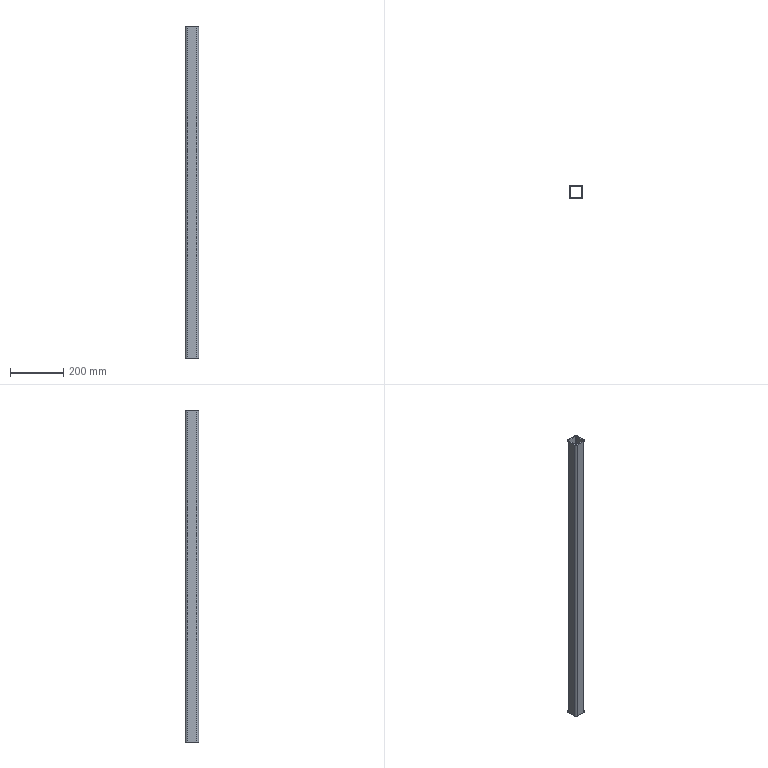Part | SolidWorks | features Extrusion 1 | 1 solid | 18 faces | box 50 x 50 x 1250 mm | volume 868496 mm3 | plane 10 | cylinder 8 | commonest cylinder face diameters 8 x4 16 x4
STEP:
#1=CARTESIAN_POINT('',(17.,-25.,625.));
#2=VERTEX_POINT('',#1);
#3=CARTESIAN_POINT('',(25.,-17.,625.));
#4=VERTEX_POINT('',#3);
#5=CARTESIAN_POINT('',(17.,-17.,625.));
#6=DIRECTION('',(0.,0.,1.));
#7=DIRECTION('',(1.,0.,0.));
#8=AXIS2_PLACEMENT_3D('',#5,#6,#7);
#9=CIRCLE('',#8,8.);
#10=EDGE_CURVE('',#2,#4,#9,.T.);
#11=ORIENTED_EDGE('',*,*,#10,.T.);
#12=CARTESIAN_POINT('',(25.,17.,625.));
#13=VERTEX_POINT('',#12);
#14=CARTESIAN_POINT('',(25.,-17.,625.));
#15=DIRECTION('',(0.,1.,0.));
#16=VECTOR('',#15,1000.);
#17=LINE('',#14,#16);
#18=EDGE_CURVE('',#4,#13,#17,.T.);
#19=ORIENTED_EDGE('',*,*,#18,.T.);
#20=CARTESIAN_POINT('',(17.,25.,625.));
#21=VERTEX_POINT('',#20);
#22=CARTESIAN_POINT('',(17.,17.,625.));
#23=DIRECTION('',(0.,0.,1.));
#24=DIRECTION('',(-1.,0.,0.));
#25=AXIS2_PLACEMENT_3D('',#22,#23,#24);
#26=CIRCLE('',#25,8.);
#27=EDGE_CURVE('',#13,#21,#26,.T.);
#28=ORIENTED_EDGE('',*,*,#27,.T.);
#29=CARTESIAN_POINT('',(-17.,25.,625.));
#30=VERTEX_POINT('',#29);
#31=CARTESIAN_POINT('',(-17.,25.,625.));
#32=DIRECTION('',(-1.,0.,0.));
#33=VECTOR('',#32,1000.);
#34=LINE('',#31,#33);
#35=EDGE_CURVE('',#21,#30,#34,.T.);
#36=ORIENTED_EDGE('',*,*,#35,.T.);
#37=CARTESIAN_POINT('',(-25.,17.,625.));
#38=VERTEX_POINT('',#37);
#39=CARTESIAN_POINT('',(-17.,17.,625.));
#40=DIRECTION('',(0.,0.,1.));
#41=DIRECTION('',(-1.,0.,0.));
#42=AXIS2_PLACEMENT_3D('',#39,#40,#41);
#43=CIRCLE('',#42,8.);
#44=EDGE_CURVE('',#30,#38,#43,.T.);
#45=ORIENTED_EDGE('',*,*,#44,.T.);
#46=CARTESIAN_POINT('',(-25.,-17.,625.));
#47=VERTEX_POINT('',#46);
#48=CARTESIAN_POINT('',(-25.,-17.,625.));
#49=DIRECTION('',(0.,-1.,0.));
#50=VECTOR('',#49,1000.);
#51=LINE('',#48,#50);
#52=EDGE_CURVE('',#38,#47,#51,.T.);
#53=ORIENTED_EDGE('',*,*,#52,.T.);
#54=CARTESIAN_POINT('',(-17.,-25.,625.));
#55=VERTEX_POINT('',#54);
#56=CARTESIAN_POINT('',(-17.,-17.,625.));
#57=DIRECTION('',(0.,0.,1.));
#58=DIRECTION('',(-1.,0.,0.));
#59=AXIS2_PLACEMENT_3D('',#56,#57,#58);
#60=CIRCLE('',#59,8.);
#61=EDGE_CURVE('',#47,#55,#60,.T.);
#62=ORIENTED_EDGE('',*,*,#61,.T.);
#63=CARTESIAN_POINT('',(-17.,-25.,625.));
#64=DIRECTION('',(1.,0.,0.));
#65=VECTOR('',#64,1000.);
#66=LINE('',#63,#65);
#67=EDGE_CURVE('',#55,#2,#66,.T.);
#68=ORIENTED_EDGE('',*,*,#67,.T.);
#69=EDGE_LOOP('',(#11,#19,#28,#36,#45,#53,#62,#68));
#70=FACE_OUTER_BOUND('',#69,.T.);
#71=CARTESIAN_POINT('',(-21.,17.,625.));
#72=VERTEX_POINT('',#71);
#73=CARTESIAN_POINT('',(-21.,-17.,625.));
#74=VERTEX_POINT('',#73);
#75=CARTESIAN_POINT('',(-21.,-17.,625.));
#76=DIRECTION('',(0.,-1.,0.));
#77=VECTOR('',#76,1000.);
#78=LINE('',#75,#77);
#79=EDGE_CURVE('',#72,#74,#78,.T.);
#80=ORIENTED_EDGE('',*,*,#79,.F.);
#81=CARTESIAN_POINT('',(-17.,21.,625.));
#82=VERTEX_POINT('',#81);
#83=CARTESIAN_POINT('',(-17.,17.,625.));
#84=DIRECTION('',(0.,0.,1.));
#85=DIRECTION('',(-1.,0.,0.));
#86=AXIS2_PLACEMENT_3D('',#83,#84,#85);
#87=CIRCLE('',#86,4.);
#88=EDGE_CURVE('',#82,#72,#87,.T.);
#89=ORIENTED_EDGE('',*,*,#88,.F.);
#90=CARTESIAN_POINT('',(17.,21.,625.));
#91=VERTEX_POINT('',#90);
#92=CARTESIAN_POINT('',(-17.,21.,625.));
#93=DIRECTION('',(-1.,0.,0.));
#94=VECTOR('',#93,1000.);
#95=LINE('',#92,#94);
#96=EDGE_CURVE('',#91,#82,#95,.T.);
#97=ORIENTED_EDGE('',*,*,#96,.F.);
#98=CARTESIAN_POINT('',(21.,17.,625.));
#99=VERTEX_POINT('',#98);
#100=CARTESIAN_POINT('',(17.,17.,625.));
#101=DIRECTION('',(0.,0.,1.));
#102=DIRECTION('',(-1.,0.,0.));
#103=AXIS2_PLACEMENT_3D('',#100,#101,#102);
#104=CIRCLE('',#103,4.);
#105=EDGE_CURVE('',#99,#91,#104,.T.);
#106=ORIENTED_EDGE('',*,*,#105,.F.);
#107=CARTESIAN_POINT('',(21.,-17.,625.));
#108=VERTEX_POINT('',#107);
#109=CARTESIAN_POINT('',(21.,-17.,625.));
#110=DIRECTION('',(0.,1.,0.));
#111=VECTOR('',#110,1000.);
#112=LINE('',#109,#111);
#113=EDGE_CURVE('',#108,#99,#112,.T.);
#114=ORIENTED_EDGE('',*,*,#113,.F.);
#115=CARTESIAN_POINT('',(17.,-21.,625.));
#116=VERTEX_POINT('',#115);
#117=CARTESIAN_POINT('',(17.,-17.,625.));
#118=DIRECTION('',(0.,0.,1.));
#119=DIRECTION('',(1.,0.,0.));
#120=AXIS2_PLACEMENT_3D('',#117,#118,#119);
#121=CIRCLE('',#120,4.);
#122=EDGE_CURVE('',#116,#108,#121,.T.);
#123=ORIENTED_EDGE('',*,*,#122,.F.);
#124=CARTESIAN_POINT('',(-17.,-21.,625.));
#125=VERTEX_POINT('',#124);
#126=CARTESIAN_POINT('',(-17.,-21.,625.));
#127=DIRECTION('',(1.,0.,0.));
#128=VECTOR('',#127,1000.);
#129=LINE('',#126,#128);
#130=EDGE_CURVE('',#125,#116,#129,.T.);
#131=ORIENTED_EDGE('',*,*,#130,.F.);
#132=CARTESIAN_POINT('',(-17.,-17.,625.));
#133=DIRECTION('',(0.,0.,1.));
#134=DIRECTION('',(-1.,0.,0.));
#135=AXIS2_PLACEMENT_3D('',#132,#133,#134);
#136=CIRCLE('',#135,4.);
#137=EDGE_CURVE('',#74,#125,#136,.T.);
#138=ORIENTED_EDGE('',*,*,#137,.F.);
#139=EDGE_LOOP('',(#80,#89,#97,#106,#114,#123,#131,#138));
#140=FACE_BOUND('',#139,.T.);
#141=CARTESIAN_POINT('',(17.,-17.,625.));
#142=DIRECTION('',(0.,0.,1.));
#143=DIRECTION('',(1.,0.,0.));
#144=AXIS2_PLACEMENT_3D('',#141,#142,#143);
#145=PLANE('',#144);
#146=ADVANCED_FACE('',(#70,#140),#145,.T.);
#147=CARTESIAN_POINT('',(17.,-25.,-625.));
#148=VERTEX_POINT('',#147);
#149=CARTESIAN_POINT('',(25.,-17.,-625.));
#150=VERTEX_POINT('',#149);
#151=CARTESIAN_POINT('',(17.,-17.,-625.));
#152=DIRECTION('',(0.,0.,1.));
#153=DIRECTION('',(1.,0.,0.));
#154=AXIS2_PLACEMENT_3D('',#151,#152,#153);
#155=CIRCLE('',#154,8.);
#156=EDGE_CURVE('',#148,#150,#155,.T.);
#157=ORIENTED_EDGE('',*,*,#156,.F.);
#158=CARTESIAN_POINT('',(-17.,-25.,-625.));
#159=VERTEX_POINT('',#158);
#160=CARTESIAN_POINT('',(-17.,-25.,-625.));
#161=DIRECTION('',(1.,0.,0.));
#162=VECTOR('',#161,1000.);
#163=LINE('',#160,#162);
#164=EDGE_CURVE('',#159,#148,#163,.T.);
#165=ORIENTED_EDGE('',*,*,#164,.F.);
#166=CARTESIAN_POINT('',(-25.,-17.,-625.));
#167=VERTEX_POINT('',#166);
#168=CARTESIAN_POINT('',(-17.,-17.,-625.));
#169=DIRECTION('',(0.,0.,1.));
#170=DIRECTION('',(-1.,0.,0.));
#171=AXIS2_PLACEMENT_3D('',#168,#169,#170);
#172=CIRCLE('',#171,8.);
#173=EDGE_CURVE('',#167,#159,#172,.T.);
#174=ORIENTED_EDGE('',*,*,#173,.F.);
#175=CARTESIAN_POINT('',(-25.,17.,-625.));
#176=VERTEX_POINT('',#175);
#177=CARTESIAN_POINT('',(-25.,-17.,-625.));
#178=DIRECTION('',(0.,-1.,0.));
#179=VECTOR('',#178,1000.);
#180=LINE('',#177,#179);
#181=EDGE_CURVE('',#176,#167,#180,.T.);
#182=ORIENTED_EDGE('',*,*,#181,.F.);
#183=CARTESIAN_POINT('',(-17.,25.,-625.));
#184=VERTEX_POINT('',#183);
#185=CARTESIAN_POINT('',(-17.,17.,-625.));
#186=DIRECTION('',(0.,0.,1.));
#187=DIRECTION('',(-1.,0.,0.));
#188=AXIS2_PLACEMENT_3D('',#185,#186,#187);
#189=CIRCLE('',#188,8.);
#190=EDGE_CURVE('',#184,#176,#189,.T.);
#191=ORIENTED_EDGE('',*,*,#190,.F.);
#192=CARTESIAN_POINT('',(17.,25.,-625.));
#193=VERTEX_POINT('',#192);
#194=CARTESIAN_POINT('',(-17.,25.,-625.));
#195=DIRECTION('',(-1.,0.,0.));
#196=VECTOR('',#195,1000.);
#197=LINE('',#194,#196);
#198=EDGE_CURVE('',#193,#184,#197,.T.);
#199=ORIENTED_EDGE('',*,*,#198,.F.);
#200=CARTESIAN_POINT('',(25.,17.,-625.));
#201=VERTEX_POINT('',#200);
#202=CARTESIAN_POINT('',(17.,17.,-625.));
#203=DIRECTION('',(0.,0.,1.));
#204=DIRECTION('',(-1.,0.,0.));
#205=AXIS2_PLACEMENT_3D('',#202,#203,#204);
#206=CIRCLE('',#205,8.);
#207=EDGE_CURVE('',#201,#193,#206,.T.);
#208=ORIENTED_EDGE('',*,*,#207,.F.);
#209=CARTESIAN_POINT('',(25.,-17.,-625.));
#210=DIRECTION('',(0.,1.,0.));
#211=VECTOR('',#210,1000.);
#212=LINE('',#209,#211);
#213=EDGE_CURVE('',#150,#201,#212,.T.);
#214=ORIENTED_EDGE('',*,*,#213,.F.);
#215=EDGE_LOOP('',(#157,#165,#174,#182,#191,#199,#208,#214));
#216=FACE_OUTER_BOUND('',#215,.T.);
#217=CARTESIAN_POINT('',(-17.,21.,-625.));
#218=VERTEX_POINT('',#217);
#219=CARTESIAN_POINT('',(-21.,17.,-625.));
#220=VERTEX_POINT('',#219);
#221=CARTESIAN_POINT('',(-17.,17.,-625.));
#222=DIRECTION('',(0.,0.,1.));
#223=DIRECTION('',(-1.,0.,0.));
#224=AXIS2_PLACEMENT_3D('',#221,#222,#223);
#225=CIRCLE('',#224,4.);
#226=EDGE_CURVE('',#218,#220,#225,.T.);
#227=ORIENTED_EDGE('',*,*,#226,.T.);
#228=CARTESIAN_POINT('',(-21.,-17.,-625.));
#229=VERTEX_POINT('',#228);
#230=CARTESIAN_POINT('',(-21.,-17.,-625.));
#231=DIRECTION('',(0.,-1.,0.));
#232=VECTOR('',#231,1000.);
#233=LINE('',#230,#232);
#234=EDGE_CURVE('',#220,#229,#233,.T.);
#235=ORIENTED_EDGE('',*,*,#234,.T.);
#236=CARTESIAN_POINT('',(-17.,-21.,-625.));
#237=VERTEX_POINT('',#236);
#238=CARTESIAN_POINT('',(-17.,-17.,-625.));
#239=DIRECTION('',(0.,0.,1.));
#240=DIRECTION('',(-1.,0.,0.));
#241=AXIS2_PLACEMENT_3D('',#238,#239,#240);
#242=CIRCLE('',#241,4.);
#243=EDGE_CURVE('',#229,#237,#242,.T.);
#244=ORIENTED_EDGE('',*,*,#243,.T.);
#245=CARTESIAN_POINT('',(17.,-21.,-625.));
#246=VERTEX_POINT('',#245);
#247=CARTESIAN_POINT('',(-17.,-21.,-625.));
#248=DIRECTION('',(1.,0.,0.));
#249=VECTOR('',#248,1000.);
#250=LINE('',#247,#249);
#251=EDGE_CURVE('',#237,#246,#250,.T.);
#252=ORIENTED_EDGE('',*,*,#251,.T.);
#253=CARTESIAN_POINT('',(21.,-17.,-625.));
#254=VERTEX_POINT('',#253);
#255=CARTESIAN_POINT('',(17.,-17.,-625.));
#256=DIRECTION('',(0.,0.,1.));
#257=DIRECTION('',(1.,0.,0.));
#258=AXIS2_PLACEMENT_3D('',#255,#256,#257);
#259=CIRCLE('',#258,4.);
#260=EDGE_CURVE('',#246,#254,#259,.T.);
#261=ORIENTED_EDGE('',*,*,#260,.T.);
#262=CARTESIAN_POINT('',(21.,17.,-625.));
#263=VERTEX_POINT('',#262);
#264=CARTESIAN_POINT('',(21.,-17.,-625.));
#265=DIRECTION('',(0.,1.,0.));
#266=VECTOR('',#265,1000.);
#267=LINE('',#264,#266);
#268=EDGE_CURVE('',#254,#263,#267,.T.);
#269=ORIENTED_EDGE('',*,*,#268,.T.);
#270=CARTESIAN_POINT('',(17.,21.,-625.));
#271=VERTEX_POINT('',#270);
#272=CARTESIAN_POINT('',(17.,17.,-625.));
#273=DIRECTION('',(0.,0.,1.));
#274=DIRECTION('',(-1.,0.,0.));
#275=AXIS2_PLACEMENT_3D('',#272,#273,#274);
#276=CIRCLE('',#275,4.);
#277=EDGE_CURVE('',#263,#271,#276,.T.);
#278=ORIENTED_EDGE('',*,*,#277,.T.);
#279=CARTESIAN_POINT('',(-17.,21.,-625.));
#280=DIRECTION('',(-1.,0.,0.));
#281=VECTOR('',#280,1000.);
#282=LINE('',#279,#281);
#283=EDGE_CURVE('',#271,#218,#282,.T.);
#284=ORIENTED_EDGE('',*,*,#283,.T.);
#285=EDGE_LOOP('',(#227,#235,#244,#252,#261,#269,#278,#284));
#286=FACE_BOUND('',#285,.T.);
#287=CARTESIAN_POINT('',(17.,-17.,-625.));
#288=DIRECTION('',(0.,0.,1.));
#289=DIRECTION('',(1.,0.,0.));
#290=AXIS2_PLACEMENT_3D('',#287,#288,#289);
#291=PLANE('',#290);
#292=ADVANCED_FACE('',(#216,#286),#291,.F.);
#293=ORIENTED_EDGE('',*,*,#156,.T.);
#294=CARTESIAN_POINT('',(25.,-17.,625.));
#295=DIRECTION('',(0.,0.,-1.));
#296=VECTOR('',#295,1000.);
#297=LINE('',#294,#296);
#298=EDGE_CURVE('',#4,#150,#297,.T.);
#299=ORIENTED_EDGE('',*,*,#298,.F.);
#300=ORIENTED_EDGE('',*,*,#10,.F.);
#301=CARTESIAN_POINT('',(17.,-25.,625.));
#302=DIRECTION('',(0.,0.,-1.));
#303=VECTOR('',#302,1000.);
#304=LINE('',#301,#303);
#305=EDGE_CURVE('',#2,#148,#304,.T.);
#306=ORIENTED_EDGE('',*,*,#305,.T.);
#307=EDGE_LOOP('',(#293,#299,#300,#306));
#308=FACE_OUTER_BOUND('',#307,.T.);
#309=CARTESIAN_POINT('',(17.,-17.,625.));
#310=DIRECTION('',(0.,0.,-1.));
#311=DIRECTION('',(-1.,0.,0.));
#312=AXIS2_PLACEMENT_3D('',#309,#310,#311);
#313=CYLINDRICAL_SURFACE('',#312,8.);
#314=ADVANCED_FACE('',(#308),#313,.T.);
#315=ORIENTED_EDGE('',*,*,#213,.T.);
#316=CARTESIAN_POINT('',(25.,17.,625.));
#317=DIRECTION('',(0.,0.,-1.));
#318=VECTOR('',#317,1000.);
#319=LINE('',#316,#318);
#320=EDGE_CURVE('',#13,#201,#319,.T.);
#321=ORIENTED_EDGE('',*,*,#320,.F.);
#322=ORIENTED_EDGE('',*,*,#18,.F.);
#323=ORIENTED_EDGE('',*,*,#298,.T.);
#324=EDGE_LOOP('',(#315,#321,#322,#323));
#325=FACE_OUTER_BOUND('',#324,.T.);
#326=CARTESIAN_POINT('',(25.,-17.,625.));
#327=DIRECTION('',(-1.,0.,0.));
#328=DIRECTION('',(0.,0.,1.));
#329=AXIS2_PLACEMENT_3D('',#326,#327,#328);
#330=PLANE('',#329);
#331=ADVANCED_FACE('',(#325),#330,.F.);
#332=ORIENTED_EDGE('',*,*,#207,.T.);
#333=CARTESIAN_POINT('',(17.,25.,625.));
#334=DIRECTION('',(0.,0.,-1.));
#335=VECTOR('',#334,1000.);
#336=LINE('',#333,#335);
#337=EDGE_CURVE('',#21,#193,#336,.T.);
#338=ORIENTED_EDGE('',*,*,#337,.F.);
#339=ORIENTED_EDGE('',*,*,#27,.F.);
#340=ORIENTED_EDGE('',*,*,#320,.T.);
#341=EDGE_LOOP('',(#332,#338,#339,#340));
#342=FACE_OUTER_BOUND('',#341,.T.);
#343=CARTESIAN_POINT('',(17.,17.,625.));
#344=DIRECTION('',(0.,0.,-1.));
#345=DIRECTION('',(-1.,0.,0.));
#346=AXIS2_PLACEMENT_3D('',#343,#344,#345);
#347=CYLINDRICAL_SURFACE('',#346,8.);
#348=ADVANCED_FACE('',(#342),#347,.T.);
#349=ORIENTED_EDGE('',*,*,#198,.T.);
#350=CARTESIAN_POINT('',(-17.,25.,625.));
#351=DIRECTION('',(0.,0.,-1.));
#352=VECTOR('',#351,1000.);
#353=LINE('',#350,#352);
#354=EDGE_CURVE('',#30,#184,#353,.T.);
#355=ORIENTED_EDGE('',*,*,#354,.F.);
#356=ORIENTED_EDGE('',*,*,#35,.F.);
#357=ORIENTED_EDGE('',*,*,#337,.T.);
#358=EDGE_LOOP('',(#349,#355,#356,#357));
#359=FACE_OUTER_BOUND('',#358,.T.);
#360=CARTESIAN_POINT('',(-17.,25.,625.));
#361=DIRECTION('',(0.,-1.,0.));
#362=DIRECTION('',(0.,0.,-1.));
#363=AXIS2_PLACEMENT_3D('',#360,#361,#362);
#364=PLANE('',#363);
#365=ADVANCED_FACE('',(#359),#364,.F.);
#366=ORIENTED_EDGE('',*,*,#190,.T.);
#367=CARTESIAN_POINT('',(-25.,17.,625.));
#368=DIRECTION('',(0.,0.,-1.));
#369=VECTOR('',#368,1000.);
#370=LINE('',#367,#369);
#371=EDGE_CURVE('',#38,#176,#370,.T.);
#372=ORIENTED_EDGE('',*,*,#371,.F.);
#373=ORIENTED_EDGE('',*,*,#44,.F.);
#374=ORIENTED_EDGE('',*,*,#354,.T.);
#375=EDGE_LOOP('',(#366,#372,#373,#374));
#376=FACE_OUTER_BOUND('',#375,.T.);
#377=CARTESIAN_POINT('',(-17.,17.,625.));
#378=DIRECTION('',(0.,0.,-1.));
#379=DIRECTION('',(-1.,0.,0.));
#380=AXIS2_PLACEMENT_3D('',#377,#378,#379);
#381=CYLINDRICAL_SURFACE('',#380,8.);
#382=ADVANCED_FACE('',(#376),#381,.T.);
#383=ORIENTED_EDGE('',*,*,#181,.T.);
#384=CARTESIAN_POINT('',(-25.,-17.,625.));
#385=DIRECTION('',(0.,0.,-1.));
#386=VECTOR('',#385,1000.);
#387=LINE('',#384,#386);
#388=EDGE_CURVE('',#47,#167,#387,.T.);
#389=ORIENTED_EDGE('',*,*,#388,.F.);
#390=ORIENTED_EDGE('',*,*,#52,.F.);
#391=ORIENTED_EDGE('',*,*,#371,.T.);
#392=EDGE_LOOP('',(#383,#389,#390,#391));
#393=FACE_OUTER_BOUND('',#392,.T.);
#394=CARTESIAN_POINT('',(-25.,-17.,625.));
#395=DIRECTION('',(1.,0.,0.));
#396=DIRECTION('',(0.,0.,-1.));
#397=AXIS2_PLACEMENT_3D('',#394,#395,#396);
#398=PLANE('',#397);
#399=ADVANCED_FACE('',(#393),#398,.F.);
#400=ORIENTED_EDGE('',*,*,#173,.T.);
#401=CARTESIAN_POINT('',(-17.,-25.,625.));
#402=DIRECTION('',(0.,0.,-1.));
#403=VECTOR('',#402,1000.);
#404=LINE('',#401,#403);
#405=EDGE_CURVE('',#55,#159,#404,.T.);
#406=ORIENTED_EDGE('',*,*,#405,.F.);
#407=ORIENTED_EDGE('',*,*,#61,.F.);
#408=ORIENTED_EDGE('',*,*,#388,.T.);
#409=EDGE_LOOP('',(#400,#406,#407,#408));
#410=FACE_OUTER_BOUND('',#409,.T.);
#411=CARTESIAN_POINT('',(-17.,-17.,625.));
#412=DIRECTION('',(0.,0.,-1.));
#413=DIRECTION('',(-1.,0.,0.));
#414=AXIS2_PLACEMENT_3D('',#411,#412,#413);
#415=CYLINDRICAL_SURFACE('',#414,8.);
#416=ADVANCED_FACE('',(#410),#415,.T.);
#417=ORIENTED_EDGE('',*,*,#164,.T.);
#418=ORIENTED_EDGE('',*,*,#305,.F.);
#419=ORIENTED_EDGE('',*,*,#67,.F.);
#420=ORIENTED_EDGE('',*,*,#405,.T.);
#421=EDGE_LOOP('',(#417,#418,#419,#420));
#422=FACE_OUTER_BOUND('',#421,.T.);
#423=CARTESIAN_POINT('',(-17.,-25.,625.));
#424=DIRECTION('',(0.,1.,0.));
#425=DIRECTION('',(0.,0.,1.));
#426=AXIS2_PLACEMENT_3D('',#423,#424,#425);
#427=PLANE('',#426);
#428=ADVANCED_FACE('',(#422),#427,.F.);
#429=ORIENTED_EDGE('',*,*,#226,.F.);
#430=CARTESIAN_POINT('',(-17.,21.,625.));
#431=DIRECTION('',(0.,0.,-1.));
#432=VECTOR('',#431,1000.);
#433=LINE('',#430,#432);
#434=EDGE_CURVE('',#82,#218,#433,.T.);
#435=ORIENTED_EDGE('',*,*,#434,.F.);
#436=ORIENTED_EDGE('',*,*,#88,.T.);
#437=CARTESIAN_POINT('',(-21.,17.,625.));
#438=DIRECTION('',(0.,0.,-1.));
#439=VECTOR('',#438,1000.);
#440=LINE('',#437,#439);
#441=EDGE_CURVE('',#72,#220,#440,.T.);
#442=ORIENTED_EDGE('',*,*,#441,.T.);
#443=EDGE_LOOP('',(#429,#435,#436,#442));
#444=FACE_OUTER_BOUND('',#443,.T.);
#445=CARTESIAN_POINT('',(-17.,17.,625.));
#446=DIRECTION('',(0.,0.,-1.));
#447=DIRECTION('',(-1.,0.,0.));
#448=AXIS2_PLACEMENT_3D('',#445,#446,#447);
#449=CYLINDRICAL_SURFACE('',#448,4.);
#450=ADVANCED_FACE('',(#444),#449,.F.);
#451=ORIENTED_EDGE('',*,*,#234,.F.);
#452=ORIENTED_EDGE('',*,*,#441,.F.);
#453=ORIENTED_EDGE('',*,*,#79,.T.);
#454=CARTESIAN_POINT('',(-21.,-17.,625.));
#455=DIRECTION('',(0.,0.,-1.));
#456=VECTOR('',#455,1000.);
#457=LINE('',#454,#456);
#458=EDGE_CURVE('',#74,#229,#457,.T.);
#459=ORIENTED_EDGE('',*,*,#458,.T.);
#460=EDGE_LOOP('',(#451,#452,#453,#459));
#461=FACE_OUTER_BOUND('',#460,.T.);
#462=CARTESIAN_POINT('',(-21.,-17.,625.));
#463=DIRECTION('',(1.,0.,0.));
#464=DIRECTION('',(0.,0.,-1.));
#465=AXIS2_PLACEMENT_3D('',#462,#463,#464);
#466=PLANE('',#465);
#467=ADVANCED_FACE('',(#461),#466,.T.);
#468=ORIENTED_EDGE('',*,*,#243,.F.);
#469=ORIENTED_EDGE('',*,*,#458,.F.);
#470=ORIENTED_EDGE('',*,*,#137,.T.);
#471=CARTESIAN_POINT('',(-17.,-21.,625.));
#472=DIRECTION('',(0.,0.,-1.));
#473=VECTOR('',#472,1000.);
#474=LINE('',#471,#473);
#475=EDGE_CURVE('',#125,#237,#474,.T.);
#476=ORIENTED_EDGE('',*,*,#475,.T.);
#477=EDGE_LOOP('',(#468,#469,#470,#476));
#478=FACE_OUTER_BOUND('',#477,.T.);
#479=CARTESIAN_POINT('',(-17.,-17.,625.));
#480=DIRECTION('',(0.,0.,-1.));
#481=DIRECTION('',(-1.,0.,0.));
#482=AXIS2_PLACEMENT_3D('',#479,#480,#481);
#483=CYLINDRICAL_SURFACE('',#482,4.);
#484=ADVANCED_FACE('',(#478),#483,.F.);
#485=ORIENTED_EDGE('',*,*,#251,.F.);
#486=ORIENTED_EDGE('',*,*,#475,.F.);
#487=ORIENTED_EDGE('',*,*,#130,.T.);
#488=CARTESIAN_POINT('',(17.,-21.,625.));
#489=DIRECTION('',(0.,0.,-1.));
#490=VECTOR('',#489,1000.);
#491=LINE('',#488,#490);
#492=EDGE_CURVE('',#116,#246,#491,.T.);
#493=ORIENTED_EDGE('',*,*,#492,.T.);
#494=EDGE_LOOP('',(#485,#486,#487,#493));
#495=FACE_OUTER_BOUND('',#494,.T.);
#496=CARTESIAN_POINT('',(-17.,-21.,625.));
#497=DIRECTION('',(0.,1.,0.));
#498=DIRECTION('',(0.,0.,1.));
#499=AXIS2_PLACEMENT_3D('',#496,#497,#498);
#500=PLANE('',#499);
#501=ADVANCED_FACE('',(#495),#500,.T.);
#502=ORIENTED_EDGE('',*,*,#260,.F.);
#503=ORIENTED_EDGE('',*,*,#492,.F.);
#504=ORIENTED_EDGE('',*,*,#122,.T.);
#505=CARTESIAN_POINT('',(21.,-17.,625.));
#506=DIRECTION('',(0.,0.,-1.));
#507=VECTOR('',#506,1000.);
#508=LINE('',#505,#507);
#509=EDGE_CURVE('',#108,#254,#508,.T.);
#510=ORIENTED_EDGE('',*,*,#509,.T.);
#511=EDGE_LOOP('',(#502,#503,#504,#510));
#512=FACE_OUTER_BOUND('',#511,.T.);
#513=CARTESIAN_POINT('',(17.,-17.,625.));
#514=DIRECTION('',(0.,0.,-1.));
#515=DIRECTION('',(-1.,0.,0.));
#516=AXIS2_PLACEMENT_3D('',#513,#514,#515);
#517=CYLINDRICAL_SURFACE('',#516,4.);
#518=ADVANCED_FACE('',(#512),#517,.F.);
#519=ORIENTED_EDGE('',*,*,#268,.F.);
#520=ORIENTED_EDGE('',*,*,#509,.F.);
#521=ORIENTED_EDGE('',*,*,#113,.T.);
#522=CARTESIAN_POINT('',(21.,17.,625.));
#523=DIRECTION('',(0.,0.,-1.));
#524=VECTOR('',#523,1000.);
#525=LINE('',#522,#524);
#526=EDGE_CURVE('',#99,#263,#525,.T.);
#527=ORIENTED_EDGE('',*,*,#526,.T.);
#528=EDGE_LOOP('',(#519,#520,#521,#527));
#529=FACE_OUTER_BOUND('',#528,.T.);
#530=CARTESIAN_POINT('',(21.,-17.,625.));
#531=DIRECTION('',(-1.,0.,0.));
#532=DIRECTION('',(0.,0.,1.));
#533=AXIS2_PLACEMENT_3D('',#530,#531,#532);
#534=PLANE('',#533);
#535=ADVANCED_FACE('',(#529),#534,.T.);
#536=ORIENTED_EDGE('',*,*,#277,.F.);
#537=ORIENTED_EDGE('',*,*,#526,.F.);
#538=ORIENTED_EDGE('',*,*,#105,.T.);
#539=CARTESIAN_POINT('',(17.,21.,625.));
#540=DIRECTION('',(0.,0.,-1.));
#541=VECTOR('',#540,1000.);
#542=LINE('',#539,#541);
#543=EDGE_CURVE('',#91,#271,#542,.T.);
#544=ORIENTED_EDGE('',*,*,#543,.T.);
#545=EDGE_LOOP('',(#536,#537,#538,#544));
#546=FACE_OUTER_BOUND('',#545,.T.);
#547=CARTESIAN_POINT('',(17.,17.,625.));
#548=DIRECTION('',(0.,0.,-1.));
#549=DIRECTION('',(-1.,0.,0.));
#550=AXIS2_PLACEMENT_3D('',#547,#548,#549);
#551=CYLINDRICAL_SURFACE('',#550,4.);
#552=ADVANCED_FACE('',(#546),#551,.F.);
#553=ORIENTED_EDGE('',*,*,#283,.F.);
#554=ORIENTED_EDGE('',*,*,#543,.F.);
#555=ORIENTED_EDGE('',*,*,#96,.T.);
#556=ORIENTED_EDGE('',*,*,#434,.T.);
#557=EDGE_LOOP('',(#553,#554,#555,#556));
#558=FACE_OUTER_BOUND('',#557,.T.);
#559=CARTESIAN_POINT('',(-17.,21.,625.));
#560=DIRECTION('',(0.,-1.,0.));
#561=DIRECTION('',(0.,0.,-1.));
#562=AXIS2_PLACEMENT_3D('',#559,#560,#561);
#563=PLANE('',#562);
#564=ADVANCED_FACE('',(#558),#563,.T.);
#565=CLOSED_SHELL('',(#146,#292,#314,#331,#348,#365,#382,#399,#416,#428,#450,#467,#484,#501,#518,#535,#552,#564));
#566=MANIFOLD_SOLID_BREP('',#565);
#567=CARTESIAN_POINT('',(0.,0.,0.));
#568=DIRECTION('',(0.,0.,1.));
#569=DIRECTION('',(1.,0.,0.));
#570=AXIS2_PLACEMENT_3D('',#567,#568,#569);
#571=(LENGTH_UNIT()NAMED_UNIT(*)SI_UNIT(.MILLI.,.METRE.));
#572=UNCERTAINTY_MEASURE_WITH_UNIT(LENGTH_MEASURE(0.00001),#571,'','');
#573=(NAMED_UNIT(*)PLANE_ANGLE_UNIT()SI_UNIT($,.RADIAN.));
#574=(NAMED_UNIT(*)SI_UNIT($,.STERADIAN.)SOLID_ANGLE_UNIT());
#575=(GEOMETRIC_REPRESENTATION_CONTEXT(3)GLOBAL_UNCERTAINTY_ASSIGNED_CONTEXT((#572))GLOBAL_UNIT_ASSIGNED_CONTEXT((#571,#573,#574))REPRESENTATION_CONTEXT('',''));
#576=ADVANCED_BREP_SHAPE_REPRESENTATION('',(#566,#570),#575);